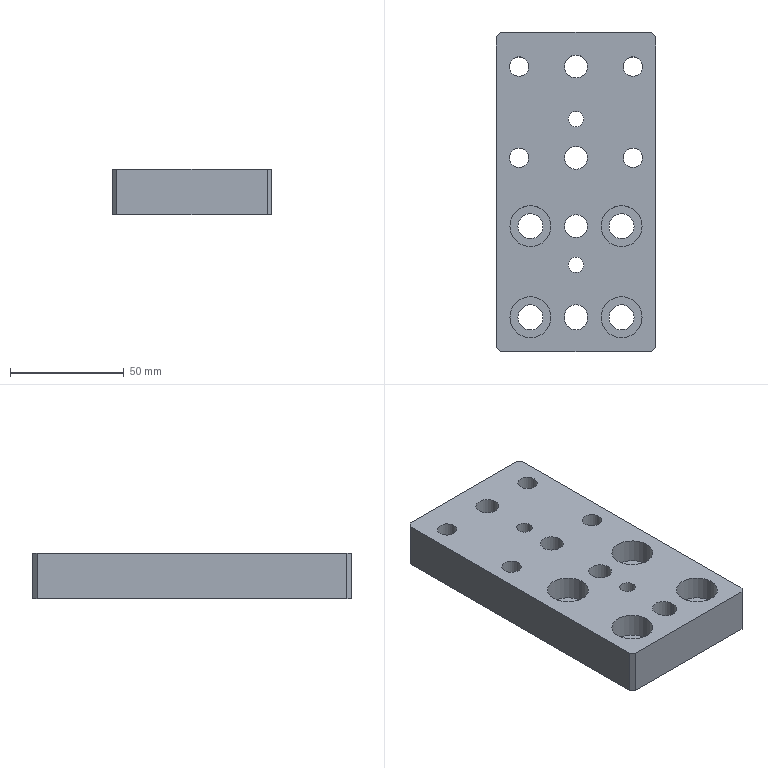CAM job | NX | 3-axis milling, drilling | part box 70 x 140 x 20 mm | stock box 70 x 140 x 20 mm
Tools:
number,name,description,diameter,corner_radius,flute_length,length,flutes
6,D6,平底铣刀-粗,6.0,0.0,25.0,75.0,2
9,D10,平底铣刀-粗,10.0,0.0,35.0,75.0,2
7,D6-J,平底铣刀-精,6.0,0.0,25.0,75.0,2
10,D10-J,平底铣刀-精,10.0,0.0,35.0,75.0,2
2,D6倒角刀,倒角刀,6.0,0.0,3.0,25.0,2
20,M8X1.25,丝锥,6.8,0.0,35.0,50.0,2
21,M10X1.5,丝锥,8.5,0.0,35.0,50.0,2
1,C6定点钻,倒角刀,6.0,0.0,3.0,3.0,2
19,ZT8.7,钻头,8.7,0.0,35.0,50.0,2
18,ZT11,钻头,11.0,0.0,35.0,50.0,2
17,ZT9.8,钻头,9.8,0.0,35.0,50.0,2
16,ZT6.9,Drilling Tool,6.9,0.0,35.0,50.0,2
Operations:
program,operation,operation_type,tool,method,geometry_group,spindle_rpm,surface_speed,feed_per_tooth,feed_cut,feed_plunge,cut_length_mm,path_length_mm,cut_time_min,machine_time_min
B,选线往复层切开粗-中_COPY_1,PlanarMilling,D10,分层开粗-切深K-步距G,W-B,3000.0,94.245,0.3333,2000.0,100.0,1832.902,2459.341,0.9165,0.9791
B,铣倒角_5,PlanarMilling,D6倒角刀,METHOD,W-B,4000.0,75.398,0.0375,300.0,100.0,47.831,233.231,0.1594,0.178
B,铣倒角_6,PlanarMilling,D6倒角刀,METHOD,W-B,3000.0,56.549,0.0667,400.0,100.0,140.605,518.905,0.3515,0.3893
B,铣倒角_7,PlanarMilling,D6倒角刀,METHOD,W-B,3000.0,56.549,0.1,600.0,100.0,112.327,353.327,0.1872,0.2113
B,铣倒角_8,PlanarMilling,D6倒角刀,METHOD,W-B,3000.0,56.549,0.1,600.0,100.0,133.995,508.698,0.2233,0.2608
B,平面去毛刺6X45L_COPY_1,SurfaceContour,D6倒角刀,爬面_倒角-切深0-步距G,W-B,3500.0,65.972,0.1429,1000.0,100.0,805.355,1512.385,0.8054,0.8761
B,平面铣精光侧面-中-直线_COPY_1,PlanarMilling,D10-J,侧刃精光-切深K-步距G,W-B,3000.0,94.245,0.1333,800.0,100.0,67.314,651.071,0.0841,0.1425
A,打点-深0.8,Operation,C6定点钻,NONE,W-A,3000.0,56.0,0.01,60.0,90.0,23.4,448.407,0.39,0.4325
A,打点-深0.8_COPY,Operation,C6定点钻,NONE,W-A,3000.0,56.0,0.01,60.0,90.0,1.8,63.6,0.03,0.0362
A,通孔-精孔10.0预钻,Operation,ZT9.8,NONE,W-A,500.0,15.394,0.12,120.0,90.0,75.987,284.003,0.6332,0.654
A,通孔-精孔10.0预钻_COPY,Operation,ZT9.8,NONE,W-A,500.0,15.394,0.12,120.0,90.0,25.329,110.658,0.2111,0.2196
A,沉头孔-钻孔0段,Operation,ZT11,NONE,W-A,500.0,17.279,0.12,120.0,90.0,105.219,393.475,0.8768,0.9057
A,通孔-M8螺纹底孔,Operation,ZT6.9,NONE,W-A,600.0,12.818,0.1,120.0,90.0,58.0,241.008,0.4833,0.5016
A,通孔-M10螺纹底孔,Operation,ZT8.7,NONE,W-A,500.0,13.352,0.12,120.0,90.0,116.0,425.035,0.9667,0.9976
A,铣倒角_1,PlanarMilling,D6倒角刀,METHOD,W-A,4000.0,75.398,0.0625,500.0,100.0,46.954,231.954,0.0939,0.1124
A,铣倒角_2,PlanarMilling,D6倒角刀,METHOD,W-A,4000.0,75.398,0.0625,500.0,100.0,137.735,516.011,0.2755,0.3133
A,铣倒角_3,PlanarMilling,D6倒角刀,METHOD,W-A,4000.0,75.398,0.0625,500.0,100.0,112.327,353.327,0.2247,0.2488
A,通孔-攻牙M8,Operation,M8X1.25,METHOD,W-A,300.0,6.409,0.0021,1.25,90.0,50.0,225.008,40.0,40.017
A,通孔-攻牙M10,Operation,M10X1.5,METHOD,W-A,200.0,5.341,0.0037,1.5,90.0,100.0,393.035,66.667,66.696
A,底壁铣螺旋开粗-中_COPY,VolumeBased25DMillingOperation,D10,分层开粗-切深K-步距G,W-A,3000.0,94.245,0.3333,2000.0,100.0,5375.151,5770.592,2.688,2.727
A,选线往复层切开粗-中_COPY,PlanarMilling,D10,分层开粗-切深K-步距G,W-A,3000.0,94.245,0.3333,2000.0,100.0,1832.902,2459.341,0.9165,0.9791
A,通腰槽粗_1,VolumeBased25DMillingOperation,D6,METHOD,W-A,3500.0,65.973,0.1714,1200.0,100.0,1968.413,2046.913,1.64,1.648
A,铣孔开粗D6_1,CylinderMilling,D6,NONE,W-A,4000.0,75.398,0.15,1200.0,100.0,3127.222,3437.222,2.606,2.637
A,铣倒角_4,PlanarMilling,D6倒角刀,NONE,W-A,4000.0,75.398,0.1,800.0,100.0,261.535,615.546,0.3269,0.3623
A,平面去毛刺6X45L_COPY,SurfaceContour,D6倒角刀,爬面_倒角-切深0-步距G,W-A,3500.0,65.972,0.1429,1000.0,100.0,1021.265,2108.226,1.021,1.13
A,底壁铣螺旋精光-中_COPY,VolumeBased25DMillingOperation,D10-J,螺旋精光-切深K-步距G,W-A,3500.0,109.952,0.1143,800.0,100.0,449.618,846.321,0.562,0.6017
A,平面铣精光侧面-中-直线_COPY,PlanarMilling,D10-J,侧刃精光-切深K-步距G,W-A,3000.0,94.245,0.1333,800.0,100.0,67.314,651.071,0.0841,0.1425
A,铣孔精光D6-J_1,CylinderMilling,D6-J,精光步距切深关,W-A,4000.0,75.398,0.05,400.0,100.0,459.437,769.437,1.149,1.18
A,腰槽精_1,VolumeBased25DMillingOperation,D6-J,METHOD,W-A,4000.0,75.398,0.05,400.0,100.0,101.813,239.746,0.2545,0.2683